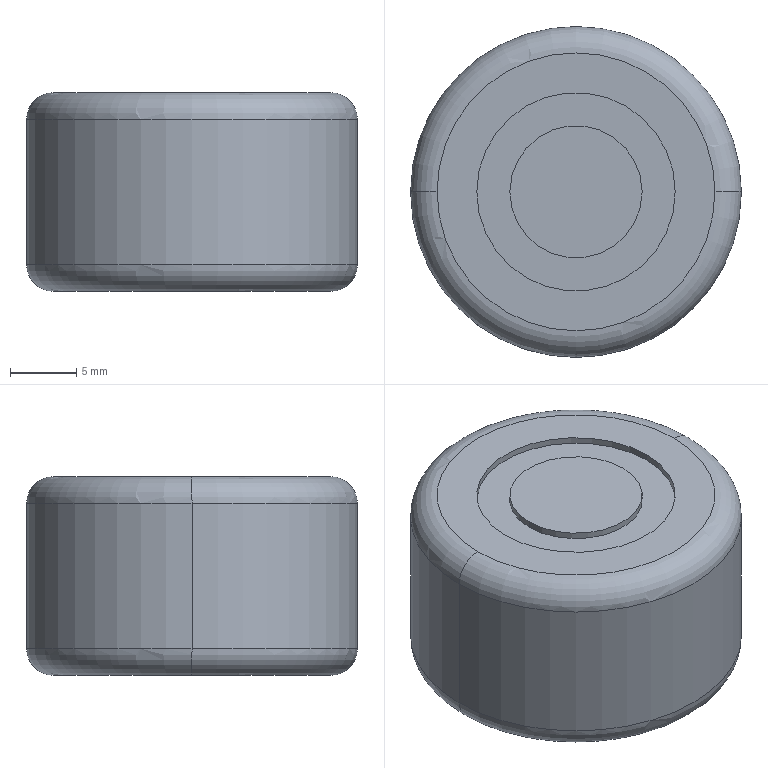Part | STEP file | Electromagnet | 1 solid | 18 faces | box 25 x 25 x 15 mm | volume 6939 mm3 | cylinder 8 | torus 4 | plane 4 | cone 2 | commonest cylinder face diameters 5 x2 10 x2 15 x2 25 x2
STEP:
#1=CARTESIAN_POINT('',(2.5,0.,12.));
#2=VERTEX_POINT('',#1);
#3=CARTESIAN_POINT('',(-2.5,0.,12.));
#4=VERTEX_POINT('',#3);
#5=CARTESIAN_POINT('',(0.,0.,12.));
#6=DIRECTION('',(0.,0.,-1.));
#7=DIRECTION('',(-1.,0.,0.));
#8=AXIS2_PLACEMENT_3D('',#5,#6,#7);
#9=CIRCLE('',#8,2.5);
#10=EDGE_CURVE('',#2,#4,#9,.T.);
#11=ORIENTED_EDGE('',*,*,#10,.F.);
#12=CARTESIAN_POINT('',(2.5,0.,0.));
#13=VERTEX_POINT('',#12);
#14=CARTESIAN_POINT('',(2.5,0.,0.));
#15=DIRECTION('',(0.,0.,-1.));
#16=VECTOR('',#15,1000.);
#17=LINE('',#14,#16);
#18=EDGE_CURVE('',#2,#13,#17,.T.);
#19=ORIENTED_EDGE('',*,*,#18,.T.);
#20=CARTESIAN_POINT('',(-2.5,0.,0.));
#21=VERTEX_POINT('',#20);
#22=CARTESIAN_POINT('',(0.,0.,0.));
#23=DIRECTION('',(0.,0.,-1.));
#24=DIRECTION('',(-1.,0.,0.));
#25=AXIS2_PLACEMENT_3D('',#22,#23,#24);
#26=CIRCLE('',#25,2.5);
#27=EDGE_CURVE('',#13,#21,#26,.T.);
#28=ORIENTED_EDGE('',*,*,#27,.T.);
#29=CARTESIAN_POINT('',(-2.5,0.,0.));
#30=DIRECTION('',(0.,0.,-1.));
#31=VECTOR('',#30,1000.);
#32=LINE('',#29,#31);
#33=EDGE_CURVE('',#4,#21,#32,.T.);
#34=ORIENTED_EDGE('',*,*,#33,.F.);
#35=EDGE_LOOP('',(#11,#19,#28,#34));
#36=FACE_OUTER_BOUND('',#35,.T.);
#37=CARTESIAN_POINT('',(0.,0.,0.));
#38=DIRECTION('',(0.,0.,-1.));
#39=DIRECTION('',(-1.,0.,0.));
#40=AXIS2_PLACEMENT_3D('',#37,#38,#39);
#41=CYLINDRICAL_SURFACE('',#40,2.5);
#42=ADVANCED_FACE('',(#36),#41,.F.);
#43=CARTESIAN_POINT('',(0.,0.,13.502));
#44=VERTEX_POINT('',#43);
#45=CARTESIAN_POINT('',(-2.5,0.,12.));
#46=DIRECTION('',(-0.8572,0.,-0.515));
#47=VECTOR('',#46,1000.);
#48=LINE('',#45,#47);
#49=EDGE_CURVE('',#44,#4,#48,.T.);
#50=ORIENTED_EDGE('',*,*,#49,.F.);
#51=CARTESIAN_POINT('',(2.5,0.,12.));
#52=DIRECTION('',(0.8572,0.,-0.515));
#53=VECTOR('',#52,1000.);
#54=LINE('',#51,#53);
#55=EDGE_CURVE('',#44,#2,#54,.T.);
#56=ORIENTED_EDGE('',*,*,#55,.T.);
#57=ORIENTED_EDGE('',*,*,#10,.T.);
#58=EDGE_LOOP('',(#50,#56,#57));
#59=FACE_OUTER_BOUND('',#58,.T.);
#60=CARTESIAN_POINT('',(0.,0.,12.));
#61=DIRECTION('',(0.,0.,-1.));
#62=DIRECTION('',(-1.,0.,0.));
#63=AXIS2_PLACEMENT_3D('',#60,#61,#62);
#64=CONICAL_SURFACE('',#63,2.5,1.03);
#65=ADVANCED_FACE('',(#59),#64,.F.);
#66=CARTESIAN_POINT('',(5.,0.,14.5));
#67=VERTEX_POINT('',#66);
#68=CARTESIAN_POINT('',(-5.,0.,14.5));
#69=VERTEX_POINT('',#68);
#70=CARTESIAN_POINT('',(0.,0.,14.5));
#71=DIRECTION('',(0.,0.,1.));
#72=DIRECTION('',(1.,0.,0.));
#73=AXIS2_PLACEMENT_3D('',#70,#71,#72);
#74=CIRCLE('',#73,5.);
#75=EDGE_CURVE('',#67,#69,#74,.T.);
#76=ORIENTED_EDGE('',*,*,#75,.T.);
#77=CARTESIAN_POINT('',(-5.,0.,15.));
#78=VERTEX_POINT('',#77);
#79=CARTESIAN_POINT('',(-5.,0.,14.5));
#80=DIRECTION('',(0.,0.,1.));
#81=VECTOR('',#80,1000.);
#82=LINE('',#79,#81);
#83=EDGE_CURVE('',#69,#78,#82,.T.);
#84=ORIENTED_EDGE('',*,*,#83,.T.);
#85=CARTESIAN_POINT('',(5.,0.,15.));
#86=VERTEX_POINT('',#85);
#87=CARTESIAN_POINT('',(0.,0.,15.));
#88=DIRECTION('',(0.,0.,1.));
#89=DIRECTION('',(1.,0.,0.));
#90=AXIS2_PLACEMENT_3D('',#87,#88,#89);
#91=CIRCLE('',#90,5.);
#92=EDGE_CURVE('',#86,#78,#91,.T.);
#93=ORIENTED_EDGE('',*,*,#92,.F.);
#94=CARTESIAN_POINT('',(5.,0.,14.5));
#95=DIRECTION('',(0.,0.,1.));
#96=VECTOR('',#95,1000.);
#97=LINE('',#94,#96);
#98=EDGE_CURVE('',#67,#86,#97,.T.);
#99=ORIENTED_EDGE('',*,*,#98,.F.);
#100=EDGE_LOOP('',(#76,#84,#93,#99));
#101=FACE_OUTER_BOUND('',#100,.T.);
#102=CARTESIAN_POINT('',(0.,0.,14.5));
#103=DIRECTION('',(0.,0.,1.));
#104=DIRECTION('',(1.,0.,0.));
#105=AXIS2_PLACEMENT_3D('',#102,#103,#104);
#106=CYLINDRICAL_SURFACE('',#105,5.);
#107=ADVANCED_FACE('',(#101),#106,.T.);
#108=CARTESIAN_POINT('',(-7.5,0.,14.5));
#109=VERTEX_POINT('',#108);
#110=CARTESIAN_POINT('',(7.5,0.,14.5));
#111=VERTEX_POINT('',#110);
#112=CARTESIAN_POINT('',(0.,0.,14.5));
#113=DIRECTION('',(0.,0.,1.));
#114=DIRECTION('',(1.,0.,0.));
#115=AXIS2_PLACEMENT_3D('',#112,#113,#114);
#116=CIRCLE('',#115,7.5);
#117=EDGE_CURVE('',#109,#111,#116,.T.);
#118=ORIENTED_EDGE('',*,*,#117,.F.);
#119=CARTESIAN_POINT('',(-7.5,0.,15.));
#120=VERTEX_POINT('',#119);
#121=CARTESIAN_POINT('',(-7.5,0.,14.5));
#122=DIRECTION('',(0.,0.,1.));
#123=VECTOR('',#122,1000.);
#124=LINE('',#121,#123);
#125=EDGE_CURVE('',#109,#120,#124,.T.);
#126=ORIENTED_EDGE('',*,*,#125,.T.);
#127=CARTESIAN_POINT('',(7.5,0.,15.));
#128=VERTEX_POINT('',#127);
#129=CARTESIAN_POINT('',(0.,0.,15.));
#130=DIRECTION('',(0.,0.,1.));
#131=DIRECTION('',(1.,0.,0.));
#132=AXIS2_PLACEMENT_3D('',#129,#130,#131);
#133=CIRCLE('',#132,7.5);
#134=EDGE_CURVE('',#120,#128,#133,.T.);
#135=ORIENTED_EDGE('',*,*,#134,.T.);
#136=CARTESIAN_POINT('',(7.5,0.,14.5));
#137=DIRECTION('',(0.,0.,1.));
#138=VECTOR('',#137,1000.);
#139=LINE('',#136,#138);
#140=EDGE_CURVE('',#111,#128,#139,.T.);
#141=ORIENTED_EDGE('',*,*,#140,.F.);
#142=EDGE_LOOP('',(#118,#126,#135,#141));
#143=FACE_OUTER_BOUND('',#142,.T.);
#144=CARTESIAN_POINT('',(0.,0.,14.5));
#145=DIRECTION('',(0.,0.,1.));
#146=DIRECTION('',(1.,0.,0.));
#147=AXIS2_PLACEMENT_3D('',#144,#145,#146);
#148=CYLINDRICAL_SURFACE('',#147,7.5);
#149=ADVANCED_FACE('',(#143),#148,.F.);
#150=CARTESIAN_POINT('',(-12.5,0.,13.));
#151=VERTEX_POINT('',#150);
#152=CARTESIAN_POINT('',(12.5,0.,13.));
#153=VERTEX_POINT('',#152);
#154=CARTESIAN_POINT('',(0.,0.,13.));
#155=DIRECTION('',(0.,0.,-1.));
#156=DIRECTION('',(1.,0.,0.));
#157=AXIS2_PLACEMENT_3D('',#154,#155,#156);
#158=CIRCLE('',#157,12.5);
#159=EDGE_CURVE('',#151,#153,#158,.T.);
#160=ORIENTED_EDGE('',*,*,#159,.F.);
#161=CARTESIAN_POINT('',(-10.5,0.,15.));
#162=VERTEX_POINT('',#161);
#163=CARTESIAN_POINT('',(-10.5,0.,13.));
#164=DIRECTION('',(0.,1.,0.));
#165=DIRECTION('',(-1.,0.,0.));
#166=AXIS2_PLACEMENT_3D('',#163,#164,#165);
#167=CIRCLE('',#166,2.);
#168=EDGE_CURVE('',#151,#162,#167,.T.);
#169=ORIENTED_EDGE('',*,*,#168,.T.);
#170=CARTESIAN_POINT('',(10.5,0.,15.));
#171=VERTEX_POINT('',#170);
#172=CARTESIAN_POINT('',(0.,0.,15.));
#173=DIRECTION('',(0.,0.,1.));
#174=DIRECTION('',(1.,0.,0.));
#175=AXIS2_PLACEMENT_3D('',#172,#173,#174);
#176=CIRCLE('',#175,10.5);
#177=EDGE_CURVE('',#171,#162,#176,.T.);
#178=ORIENTED_EDGE('',*,*,#177,.F.);
#179=CARTESIAN_POINT('',(10.5,0.,13.));
#180=DIRECTION('',(0.,-1.,0.));
#181=DIRECTION('',(0.,0.,-1.));
#182=AXIS2_PLACEMENT_3D('',#179,#180,#181);
#183=CIRCLE('',#182,2.);
#184=EDGE_CURVE('',#153,#171,#183,.T.);
#185=ORIENTED_EDGE('',*,*,#184,.F.);
#186=EDGE_LOOP('',(#160,#169,#178,#185));
#187=FACE_OUTER_BOUND('',#186,.T.);
#188=CARTESIAN_POINT('',(0.,0.,13.));
#189=DIRECTION('',(0.,0.,1.));
#190=DIRECTION('',(1.,0.,0.));
#191=AXIS2_PLACEMENT_3D('',#188,#189,#190);
#192=TOROIDAL_SURFACE('',#191,10.5,2.);
#193=ADVANCED_FACE('',(#187),#192,.T.);
#194=CARTESIAN_POINT('',(-10.5,0.,0.));
#195=VERTEX_POINT('',#194);
#196=CARTESIAN_POINT('',(10.5,0.,0.));
#197=VERTEX_POINT('',#196);
#198=CARTESIAN_POINT('',(0.,0.,0.));
#199=DIRECTION('',(0.,0.,-1.));
#200=DIRECTION('',(1.,0.,0.));
#201=AXIS2_PLACEMENT_3D('',#198,#199,#200);
#202=CIRCLE('',#201,10.5);
#203=EDGE_CURVE('',#195,#197,#202,.T.);
#204=ORIENTED_EDGE('',*,*,#203,.F.);
#205=CARTESIAN_POINT('',(-12.5,0.,2.));
#206=VERTEX_POINT('',#205);
#207=CARTESIAN_POINT('',(-10.5,0.,2.));
#208=DIRECTION('',(0.,1.,0.));
#209=DIRECTION('',(-1.,0.,0.));
#210=AXIS2_PLACEMENT_3D('',#207,#208,#209);
#211=CIRCLE('',#210,2.);
#212=EDGE_CURVE('',#195,#206,#211,.T.);
#213=ORIENTED_EDGE('',*,*,#212,.T.);
#214=CARTESIAN_POINT('',(12.5,0.,2.));
#215=VERTEX_POINT('',#214);
#216=CARTESIAN_POINT('',(0.,0.,2.));
#217=DIRECTION('',(0.,0.,1.));
#218=DIRECTION('',(1.,0.,0.));
#219=AXIS2_PLACEMENT_3D('',#216,#217,#218);
#220=CIRCLE('',#219,12.5);
#221=EDGE_CURVE('',#215,#206,#220,.T.);
#222=ORIENTED_EDGE('',*,*,#221,.F.);
#223=CARTESIAN_POINT('',(10.5,0.,2.));
#224=DIRECTION('',(0.,-1.,0.));
#225=DIRECTION('',(0.,0.,-1.));
#226=AXIS2_PLACEMENT_3D('',#223,#224,#225);
#227=CIRCLE('',#226,2.);
#228=EDGE_CURVE('',#197,#215,#227,.T.);
#229=ORIENTED_EDGE('',*,*,#228,.F.);
#230=EDGE_LOOP('',(#204,#213,#222,#229));
#231=FACE_OUTER_BOUND('',#230,.T.);
#232=CARTESIAN_POINT('',(0.,0.,2.));
#233=DIRECTION('',(0.,0.,1.));
#234=DIRECTION('',(1.,0.,0.));
#235=AXIS2_PLACEMENT_3D('',#232,#233,#234);
#236=TOROIDAL_SURFACE('',#235,10.5,2.);
#237=ADVANCED_FACE('',(#231),#236,.T.);
#238=ORIENTED_EDGE('',*,*,#159,.T.);
#239=CARTESIAN_POINT('',(12.5,0.,15.));
#240=DIRECTION('',(0.,0.,-1.));
#241=VECTOR('',#240,1000.);
#242=LINE('',#239,#241);
#243=EDGE_CURVE('',#153,#215,#242,.T.);
#244=ORIENTED_EDGE('',*,*,#243,.T.);
#245=ORIENTED_EDGE('',*,*,#221,.T.);
#246=CARTESIAN_POINT('',(-12.5,0.,15.));
#247=DIRECTION('',(0.,0.,-1.));
#248=VECTOR('',#247,1000.);
#249=LINE('',#246,#248);
#250=EDGE_CURVE('',#151,#206,#249,.T.);
#251=ORIENTED_EDGE('',*,*,#250,.F.);
#252=EDGE_LOOP('',(#238,#244,#245,#251));
#253=FACE_OUTER_BOUND('',#252,.T.);
#254=CARTESIAN_POINT('',(0.,0.,15.));
#255=DIRECTION('',(0.,0.,-1.));
#256=DIRECTION('',(-1.,0.,0.));
#257=AXIS2_PLACEMENT_3D('',#254,#255,#256);
#258=CYLINDRICAL_SURFACE('',#257,12.5);
#259=ADVANCED_FACE('',(#253),#258,.T.);
#260=ORIENTED_EDGE('',*,*,#243,.F.);
#261=CARTESIAN_POINT('',(0.,0.,13.));
#262=DIRECTION('',(0.,0.,-1.));
#263=DIRECTION('',(1.,0.,0.));
#264=AXIS2_PLACEMENT_3D('',#261,#262,#263);
#265=CIRCLE('',#264,12.5);
#266=EDGE_CURVE('',#153,#151,#265,.T.);
#267=ORIENTED_EDGE('',*,*,#266,.T.);
#268=ORIENTED_EDGE('',*,*,#250,.T.);
#269=CARTESIAN_POINT('',(0.,0.,2.));
#270=DIRECTION('',(0.,0.,1.));
#271=DIRECTION('',(1.,0.,0.));
#272=AXIS2_PLACEMENT_3D('',#269,#270,#271);
#273=CIRCLE('',#272,12.5);
#274=EDGE_CURVE('',#206,#215,#273,.T.);
#275=ORIENTED_EDGE('',*,*,#274,.T.);
#276=EDGE_LOOP('',(#260,#267,#268,#275));
#277=FACE_OUTER_BOUND('',#276,.T.);
#278=CARTESIAN_POINT('',(0.,0.,15.));
#279=DIRECTION('',(0.,0.,-1.));
#280=DIRECTION('',(-1.,0.,0.));
#281=AXIS2_PLACEMENT_3D('',#278,#279,#280);
#282=CYLINDRICAL_SURFACE('',#281,12.5);
#283=ADVANCED_FACE('',(#277),#282,.T.);
#284=CARTESIAN_POINT('',(0.,0.,15.));
#285=DIRECTION('',(0.,0.,1.));
#286=DIRECTION('',(1.,0.,0.));
#287=AXIS2_PLACEMENT_3D('',#284,#285,#286);
#288=CIRCLE('',#287,7.5);
#289=EDGE_CURVE('',#128,#120,#288,.T.);
#290=ORIENTED_EDGE('',*,*,#289,.F.);
#291=ORIENTED_EDGE('',*,*,#134,.F.);
#292=EDGE_LOOP('',(#290,#291));
#293=FACE_BOUND('',#292,.T.);
#294=ORIENTED_EDGE('',*,*,#177,.T.);
#295=CARTESIAN_POINT('',(0.,0.,15.));
#296=DIRECTION('',(0.,0.,1.));
#297=DIRECTION('',(1.,0.,0.));
#298=AXIS2_PLACEMENT_3D('',#295,#296,#297);
#299=CIRCLE('',#298,10.5);
#300=EDGE_CURVE('',#162,#171,#299,.T.);
#301=ORIENTED_EDGE('',*,*,#300,.T.);
#302=EDGE_LOOP('',(#294,#301));
#303=FACE_OUTER_BOUND('',#302,.T.);
#304=CARTESIAN_POINT('',(0.,0.,15.));
#305=DIRECTION('',(0.,0.,1.));
#306=DIRECTION('',(1.,0.,0.));
#307=AXIS2_PLACEMENT_3D('',#304,#305,#306);
#308=PLANE('',#307);
#309=ADVANCED_FACE('',(#293,#303),#308,.T.);
#310=CARTESIAN_POINT('',(0.,0.,0.));
#311=DIRECTION('',(0.,0.,-1.));
#312=DIRECTION('',(-1.,0.,0.));
#313=AXIS2_PLACEMENT_3D('',#310,#311,#312);
#314=CIRCLE('',#313,2.5);
#315=EDGE_CURVE('',#21,#13,#314,.T.);
#316=ORIENTED_EDGE('',*,*,#315,.F.);
#317=ORIENTED_EDGE('',*,*,#27,.F.);
#318=EDGE_LOOP('',(#316,#317));
#319=FACE_BOUND('',#318,.T.);
#320=CARTESIAN_POINT('',(0.,0.,0.));
#321=DIRECTION('',(0.,0.,-1.));
#322=DIRECTION('',(1.,0.,0.));
#323=AXIS2_PLACEMENT_3D('',#320,#321,#322);
#324=CIRCLE('',#323,10.5);
#325=EDGE_CURVE('',#197,#195,#324,.T.);
#326=ORIENTED_EDGE('',*,*,#325,.T.);
#327=ORIENTED_EDGE('',*,*,#203,.T.);
#328=EDGE_LOOP('',(#326,#327));
#329=FACE_OUTER_BOUND('',#328,.T.);
#330=CARTESIAN_POINT('',(0.,0.,0.));
#331=DIRECTION('',(0.,0.,1.));
#332=DIRECTION('',(1.,0.,0.));
#333=AXIS2_PLACEMENT_3D('',#330,#331,#332);
#334=PLANE('',#333);
#335=ADVANCED_FACE('',(#319,#329),#334,.F.);
#336=ORIENTED_EDGE('',*,*,#212,.F.);
#337=ORIENTED_EDGE('',*,*,#325,.F.);
#338=ORIENTED_EDGE('',*,*,#228,.T.);
#339=ORIENTED_EDGE('',*,*,#274,.F.);
#340=EDGE_LOOP('',(#336,#337,#338,#339));
#341=FACE_OUTER_BOUND('',#340,.T.);
#342=CARTESIAN_POINT('',(0.,0.,2.));
#343=DIRECTION('',(0.,0.,1.));
#344=DIRECTION('',(1.,0.,0.));
#345=AXIS2_PLACEMENT_3D('',#342,#343,#344);
#346=TOROIDAL_SURFACE('',#345,10.5,2.);
#347=ADVANCED_FACE('',(#341),#346,.T.);
#348=ORIENTED_EDGE('',*,*,#168,.F.);
#349=ORIENTED_EDGE('',*,*,#266,.F.);
#350=ORIENTED_EDGE('',*,*,#184,.T.);
#351=ORIENTED_EDGE('',*,*,#300,.F.);
#352=EDGE_LOOP('',(#348,#349,#350,#351));
#353=FACE_OUTER_BOUND('',#352,.T.);
#354=CARTESIAN_POINT('',(0.,0.,13.));
#355=DIRECTION('',(0.,0.,1.));
#356=DIRECTION('',(1.,0.,0.));
#357=AXIS2_PLACEMENT_3D('',#354,#355,#356);
#358=TOROIDAL_SURFACE('',#357,10.5,2.);
#359=ADVANCED_FACE('',(#353),#358,.T.);
#360=ORIENTED_EDGE('',*,*,#125,.F.);
#361=CARTESIAN_POINT('',(0.,0.,14.5));
#362=DIRECTION('',(0.,0.,1.));
#363=DIRECTION('',(1.,0.,0.));
#364=AXIS2_PLACEMENT_3D('',#361,#362,#363);
#365=CIRCLE('',#364,7.5);
#366=EDGE_CURVE('',#111,#109,#365,.T.);
#367=ORIENTED_EDGE('',*,*,#366,.F.);
#368=ORIENTED_EDGE('',*,*,#140,.T.);
#369=ORIENTED_EDGE('',*,*,#289,.T.);
#370=EDGE_LOOP('',(#360,#367,#368,#369));
#371=FACE_OUTER_BOUND('',#370,.T.);
#372=CARTESIAN_POINT('',(0.,0.,14.5));
#373=DIRECTION('',(0.,0.,1.));
#374=DIRECTION('',(1.,0.,0.));
#375=AXIS2_PLACEMENT_3D('',#372,#373,#374);
#376=CYLINDRICAL_SURFACE('',#375,7.5);
#377=ADVANCED_FACE('',(#371),#376,.F.);
#378=ORIENTED_EDGE('',*,*,#75,.F.);
#379=CARTESIAN_POINT('',(0.,0.,14.5));
#380=DIRECTION('',(0.,0.,1.));
#381=DIRECTION('',(1.,0.,0.));
#382=AXIS2_PLACEMENT_3D('',#379,#380,#381);
#383=CIRCLE('',#382,5.);
#384=EDGE_CURVE('',#69,#67,#383,.T.);
#385=ORIENTED_EDGE('',*,*,#384,.F.);
#386=EDGE_LOOP('',(#378,#385));
#387=FACE_BOUND('',#386,.T.);
#388=ORIENTED_EDGE('',*,*,#366,.T.);
#389=ORIENTED_EDGE('',*,*,#117,.T.);
#390=EDGE_LOOP('',(#388,#389));
#391=FACE_OUTER_BOUND('',#390,.T.);
#392=CARTESIAN_POINT('',(0.,0.,14.5));
#393=DIRECTION('',(0.,0.,1.));
#394=DIRECTION('',(1.,0.,0.));
#395=AXIS2_PLACEMENT_3D('',#392,#393,#394);
#396=PLANE('',#395);
#397=ADVANCED_FACE('',(#387,#391),#396,.T.);
#398=ORIENTED_EDGE('',*,*,#83,.F.);
#399=ORIENTED_EDGE('',*,*,#384,.T.);
#400=ORIENTED_EDGE('',*,*,#98,.T.);
#401=CARTESIAN_POINT('',(0.,0.,15.));
#402=DIRECTION('',(0.,0.,1.));
#403=DIRECTION('',(1.,0.,0.));
#404=AXIS2_PLACEMENT_3D('',#401,#402,#403);
#405=CIRCLE('',#404,5.);
#406=EDGE_CURVE('',#78,#86,#405,.T.);
#407=ORIENTED_EDGE('',*,*,#406,.F.);
#408=EDGE_LOOP('',(#398,#399,#400,#407));
#409=FACE_OUTER_BOUND('',#408,.T.);
#410=CARTESIAN_POINT('',(0.,0.,14.5));
#411=DIRECTION('',(0.,0.,1.));
#412=DIRECTION('',(1.,0.,0.));
#413=AXIS2_PLACEMENT_3D('',#410,#411,#412);
#414=CYLINDRICAL_SURFACE('',#413,5.);
#415=ADVANCED_FACE('',(#409),#414,.T.);
#416=ORIENTED_EDGE('',*,*,#92,.T.);
#417=ORIENTED_EDGE('',*,*,#406,.T.);
#418=EDGE_LOOP('',(#416,#417));
#419=FACE_OUTER_BOUND('',#418,.T.);
#420=CARTESIAN_POINT('',(0.,0.,15.));
#421=DIRECTION('',(0.,0.,1.));
#422=DIRECTION('',(1.,0.,0.));
#423=AXIS2_PLACEMENT_3D('',#420,#421,#422);
#424=PLANE('',#423);
#425=ADVANCED_FACE('',(#419),#424,.T.);
#426=ORIENTED_EDGE('',*,*,#55,.F.);
#427=ORIENTED_EDGE('',*,*,#49,.T.);
#428=CARTESIAN_POINT('',(0.,0.,12.));
#429=DIRECTION('',(0.,0.,-1.));
#430=DIRECTION('',(-1.,0.,0.));
#431=AXIS2_PLACEMENT_3D('',#428,#429,#430);
#432=CIRCLE('',#431,2.5);
#433=EDGE_CURVE('',#4,#2,#432,.T.);
#434=ORIENTED_EDGE('',*,*,#433,.T.);
#435=EDGE_LOOP('',(#426,#427,#434));
#436=FACE_OUTER_BOUND('',#435,.T.);
#437=CARTESIAN_POINT('',(0.,0.,12.));
#438=DIRECTION('',(0.,0.,-1.));
#439=DIRECTION('',(-1.,0.,0.));
#440=AXIS2_PLACEMENT_3D('',#437,#438,#439);
#441=CONICAL_SURFACE('',#440,2.5,1.03);
#442=ADVANCED_FACE('',(#436),#441,.F.);
#443=ORIENTED_EDGE('',*,*,#18,.F.);
#444=ORIENTED_EDGE('',*,*,#433,.F.);
#445=ORIENTED_EDGE('',*,*,#33,.T.);
#446=ORIENTED_EDGE('',*,*,#315,.T.);
#447=EDGE_LOOP('',(#443,#444,#445,#446));
#448=FACE_OUTER_BOUND('',#447,.T.);
#449=CARTESIAN_POINT('',(0.,0.,0.));
#450=DIRECTION('',(0.,0.,-1.));
#451=DIRECTION('',(-1.,0.,0.));
#452=AXIS2_PLACEMENT_3D('',#449,#450,#451);
#453=CYLINDRICAL_SURFACE('',#452,2.5);
#454=ADVANCED_FACE('',(#448),#453,.F.);
#455=CLOSED_SHELL('',(#42,#65,#107,#149,#193,#237,#259,#283,#309,#335,#347,#359,#377,#397,#415,#425,#442,#454));
#456=MANIFOLD_SOLID_BREP('',#455);
#457=CARTESIAN_POINT('',(0.,0.,0.));
#458=DIRECTION('',(0.,0.,1.));
#459=DIRECTION('',(1.,0.,0.));
#460=AXIS2_PLACEMENT_3D('',#457,#458,#459);
#461=(LENGTH_UNIT()NAMED_UNIT(*)SI_UNIT(.MILLI.,.METRE.));
#462=UNCERTAINTY_MEASURE_WITH_UNIT(LENGTH_MEASURE(0.00001),#461,'','');
#463=(NAMED_UNIT(*)PLANE_ANGLE_UNIT()SI_UNIT($,.RADIAN.));
#464=(NAMED_UNIT(*)SI_UNIT($,.STERADIAN.)SOLID_ANGLE_UNIT());
#465=(GEOMETRIC_REPRESENTATION_CONTEXT(3)GLOBAL_UNCERTAINTY_ASSIGNED_CONTEXT((#462))GLOBAL_UNIT_ASSIGNED_CONTEXT((#461,#463,#464))REPRESENTATION_CONTEXT('',''));
#466=ADVANCED_BREP_SHAPE_REPRESENTATION('',(#456,#460),#465);